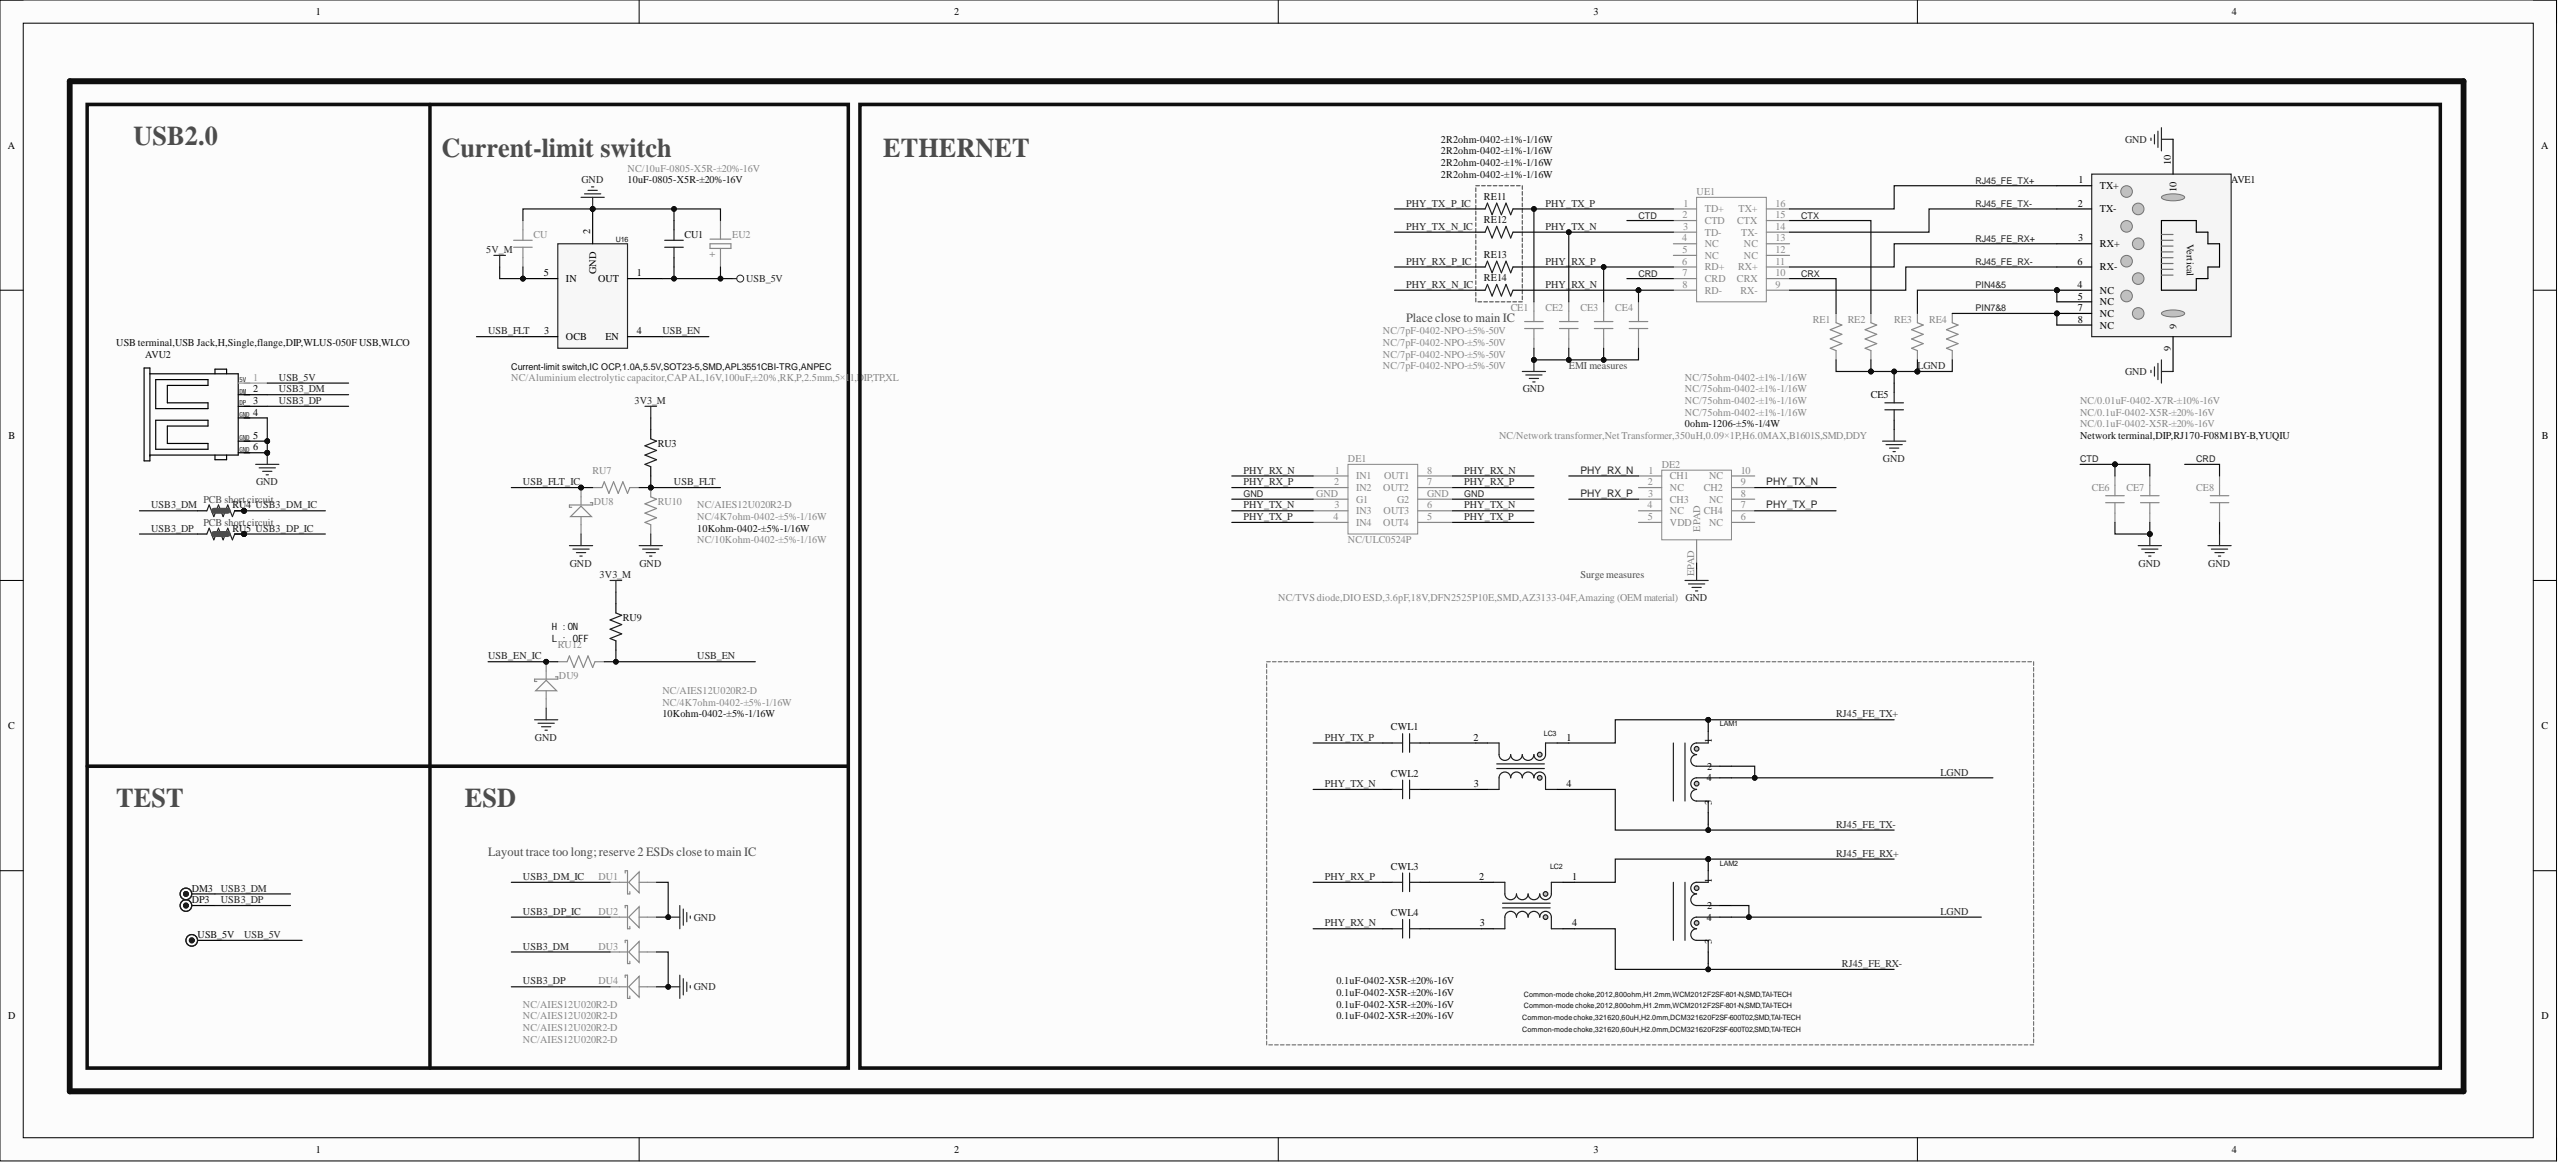Circuit board | Altium Designer | 951 parts | 509 nets | one sheet of the schematic
Parts on this sheet (reference | value | footprint):
AVE1 | Network terminal,DIP,RJ170-F08M1BY-B,YUQIU | RJ45-VD-16
AVU2 | USB terminal,USB Jack,H,Single,flange,DIP,WLUS-050F USB,WLCO | USB1-HD-2
CE1 | NC/7pF-0402-NPO-±5%-50V | C0402
CE2 | NC/7pF-0402-NPO-±5%-50V | C0402
CE3 | NC/7pF-0402-NPO-±5%-50V | C0402
CE4 | NC/7pF-0402-NPO-±5%-50V | C0402
CE5 | 0ohm-1206-±5%-1/4W | C1206
CE6 | NC/0.1uF-0402-X5R-±20%-16V | C0402
CE7 | NC/0.01uF-0402-X7R-±10%-16V | C0402
CE8 | NC/0.1uF-0402-X5R-±20%-16V | C0402
CU | NC/10uF-0805-X5R-±20%-16V | C0805
CU1 | 10uF-0805-X5R-±20%-16V | C0805
CWL2 | 0.1uF-0402-X5R-±20%-16V | C0402
CWL3 | 0.1uF-0402-X5R-±20%-16V | C0402
CWL4 | 0.1uF-0402-X5R-±20%-16V | C0402
DE1 | NC/ULC0524P | RCL0524P
DE2 | NC/TVS diode,DIO ESD,3.6pF,18V,DFN2525P10E,SMD,AZ3133-04F,Amazing (OEM material) | DFN10/0.5-2
DM3 | TEST | TP
DP3 | TEST | TP
DU1 | NC/AIES12U020R2-D | DIODE-S0402
DU2 | NC/AIES12U020R2-D | DIODE-S0402
DU3 | NC/AIES12U020R2-D | DIODE-S0402
DU4 | NC/AIES12U020R2-D | DIODE-S0402
DU8 | NC/AIES12U020R2-D | DIODE-S0402
DU9 | NC/AIES12U020R2-D | DIODE-S0402
EU2 | NC/Aluminium electrolytic capacitor,CAP AL,16V,100uF,±20%,RK,P,2.5mm,5×11,DIP,TP,XL | EC(5*11)-V-2.5
LAM1 | Common-mode choke,321620,60uH,H2.0mm,DCM321620F2SF-600T02,SMD,TAI-TECH | L/LC4/3.2*1.6
LAM2 | Common-mode choke,321620,60uH,H2.0mm,DCM321620F2SF-600T02,SMD,TAI-TECH | L/LC4/3.2*1.6
LC2 | Common-mode choke,2012,800ohm,H1.2mm,WCM2012F2SF-801-N,SMD,TAI-TECH | L/LC4/2*1.2-S
LC3 | Common-mode choke,2012,800ohm,H1.2mm,WCM2012F2SF-801-N,SMD,TAI-TECH | L/LC4/2*1.2-S
RE1 | NC/75ohm-0402-±1%-1/16W | R0402
RE2 | NC/75ohm-0402-±1%-1/16W | R0402
RE3 | NC/75ohm-0402-±1%-1/16W | R0402
RE4 | NC/75ohm-0402-±1%-1/16W | R0402
RE11 | 2R2ohm-0402-±1%-1/16W | R0402
RE12 | 2R2ohm-0402-±1%-1/16W | R0402
RE13 | 2R2ohm-0402-±1%-1/16W | R0402
RE14 | 2R2ohm-0402-±1%-1/16W | R0402
RU3 | 10Kohm-0402-±5%-1/16W | R0402
RU4 | NC/0ohm-0402-PCB | R0402SC
RU5 | NC/0ohm-0402-PCB | R0402SC
RU7 | NC/4K7ohm-0402-±5%-1/16W | R0402
RU9 | 10Kohm-0402-±5%-1/16W | R0402
RU10 | NC/10Kohm-0402-±5%-1/16W | R0402
RU12 | NC/4K7ohm-0402-±5%-1/16W | R0402
U16 | Current-limit switch,IC OCP,1.0A,5.5V,SOT23-5,SMD,APL3551CBI-TRG,ANPEC | SOT-23-5
UE1 | NC/Network transformer,Net Transformer,350uH,0.09×1P,H6.0MAX,B1601S,SMD,DDY | SOP16/1.27-2
USB_5V | TEST | TP
Nets of these parts (net: part-pin ...):
USB_FLT_IC: DU8-K RU7-1
USB_FLT: RU3-1 RU7-2 RU10-2 U16-3
USB_EN_IC: DU9-K RU12-1
USB_EN: RU9-1 RU12-2 U16-4
USB_5V: AVU2-1 CU1-2 EU2-1 U16-1 USB_5V-1
USB3_DP_IC: DU2-K RU5-2 RU5-3
USB3_DP: AVU2-3 DP3-1 DU4-K RU5-1
USB3_DM_IC: DU1-K RU4-2 RU4-3
USB3_DM: AVU2-2 DM3-1 DU3-K RU4-1
RJ45_FE_TX-: AVE1-2 LAM1-3 LC3-4 UE1-14
RJ45_FE_TX+: AVE1-1 LAM1-1 LC3-1 UE1-16
RJ45_FE_RX-: AVE1-6 LAM2-3 LC2-4 UE1-9
RJ45_FE_RX+: AVE1-3 LAM2-1 LC2-1 UE1-11
PIN7&8: AVE1-7 AVE1-8 RE4-2
PIN4&5: AVE1-4 AVE1-5 RE3-2
PHY_TX_P_IC: RE11-1
PHY_TX_P: CE1-2 DE1-4 DE1-5 DE2-7 RE11-2 UE1-1
PHY_TX_N_IC: RE12-1
PHY_TX_N: CE2-2 CWL2-1 DE1-3 DE1-6 DE2-9 RE12-2 UE1-3
PHY_RX_P_IC: RE13-1
PHY_RX_P: CE3-2 CWL3-1 DE1-2 DE1-7 DE2-3 RE13-2 UE1-6
PHY_RX_N_IC: RE14-1
PHY_RX_N: CE4-2 CWL4-1 DE1-1 DE1-8 DE2-1 RE14-2 UE1-8
NetCWL4_2: CWL4-2 LC2-3
NetCWL3_2: CWL3-2 LC2-2
NetCWL2_2: CWL2-2 LC3-3
NetCWL1_2: LC3-2
LGND: CE5-1 LAM1-2 LAM1-4 LAM2-2 LAM2-4 RE1-1 RE2-1 RE3-1 RE4-1
GND: AVE1-9 AVE1-10 AVU2-4 AVU2-5 AVU2-6 CE1-1 CE2-1 CE3-1 CE4-1 CE5-2 CE6-1 CE7-1 CE8-2 CU1-1 CU-2 DE1-GND DE2-EPAD DU1-A DU2-A DU3-A DU4-A DU8-A DU9-A EU2-2 RU10-1 U16-2
CTX: RE2-2 UE1-15
CTD: CE6-2 CE7-2 UE1-2
CRX: RE1-2 UE1-10
CRD: CE8-1 UE1-7
5V_M: CU-1 U16-5
3V3_M: RU3-2 RU9-2